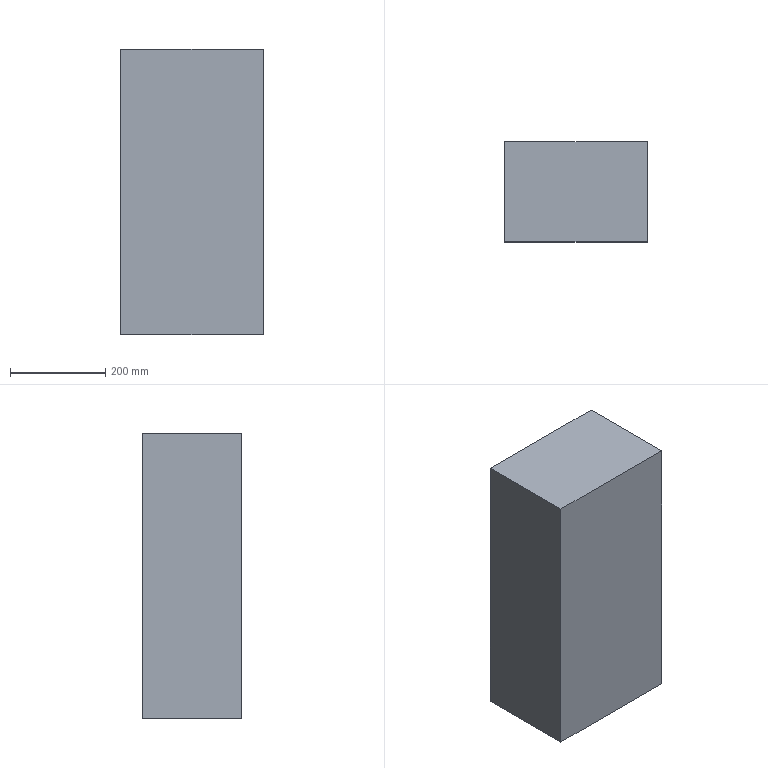Part | SolidWorks | features Extrusion 1 | 1 solid | 6 faces | box 300 x 210 x 600 mm | volume 37800000 mm3 | plane 6
STEP:
#1=CARTESIAN_POINT('',(150.,-105.,0.));
#2=VERTEX_POINT('',#1);
#3=CARTESIAN_POINT('',(150.,105.,0.));
#4=VERTEX_POINT('',#3);
#5=CARTESIAN_POINT('',(150.,105.,0.));
#6=DIRECTION('',(0.,1.,0.));
#7=VECTOR('',#6,1000.);
#8=LINE('',#5,#7);
#9=EDGE_CURVE('',#2,#4,#8,.T.);
#10=ORIENTED_EDGE('',*,*,#9,.T.);
#11=CARTESIAN_POINT('',(150.,105.,600.));
#12=VERTEX_POINT('',#11);
#13=CARTESIAN_POINT('',(150.,105.,600.));
#14=DIRECTION('',(0.,0.,-1.));
#15=VECTOR('',#14,1000.);
#16=LINE('',#13,#15);
#17=EDGE_CURVE('',#12,#4,#16,.T.);
#18=ORIENTED_EDGE('',*,*,#17,.F.);
#19=CARTESIAN_POINT('',(150.,-105.,600.));
#20=VERTEX_POINT('',#19);
#21=CARTESIAN_POINT('',(150.,105.,600.));
#22=DIRECTION('',(0.,1.,0.));
#23=VECTOR('',#22,1000.);
#24=LINE('',#21,#23);
#25=EDGE_CURVE('',#20,#12,#24,.T.);
#26=ORIENTED_EDGE('',*,*,#25,.F.);
#27=CARTESIAN_POINT('',(150.,-105.,600.));
#28=DIRECTION('',(0.,0.,-1.));
#29=VECTOR('',#28,1000.);
#30=LINE('',#27,#29);
#31=EDGE_CURVE('',#20,#2,#30,.T.);
#32=ORIENTED_EDGE('',*,*,#31,.T.);
#33=EDGE_LOOP('',(#10,#18,#26,#32));
#34=FACE_OUTER_BOUND('',#33,.T.);
#35=CARTESIAN_POINT('',(150.,105.,600.));
#36=DIRECTION('',(-1.,0.,0.));
#37=DIRECTION('',(0.,0.,1.));
#38=AXIS2_PLACEMENT_3D('',#35,#36,#37);
#39=PLANE('',#38);
#40=ADVANCED_FACE('',(#34),#39,.F.);
#41=CARTESIAN_POINT('',(-150.,105.,0.));
#42=VERTEX_POINT('',#41);
#43=CARTESIAN_POINT('',(-150.,105.,0.));
#44=DIRECTION('',(-1.,0.,0.));
#45=VECTOR('',#44,1000.);
#46=LINE('',#43,#45);
#47=EDGE_CURVE('',#4,#42,#46,.T.);
#48=ORIENTED_EDGE('',*,*,#47,.T.);
#49=CARTESIAN_POINT('',(-150.,105.,600.));
#50=VERTEX_POINT('',#49);
#51=CARTESIAN_POINT('',(-150.,105.,600.));
#52=DIRECTION('',(0.,0.,-1.));
#53=VECTOR('',#52,1000.);
#54=LINE('',#51,#53);
#55=EDGE_CURVE('',#50,#42,#54,.T.);
#56=ORIENTED_EDGE('',*,*,#55,.F.);
#57=CARTESIAN_POINT('',(-150.,105.,600.));
#58=DIRECTION('',(-1.,0.,0.));
#59=VECTOR('',#58,1000.);
#60=LINE('',#57,#59);
#61=EDGE_CURVE('',#12,#50,#60,.T.);
#62=ORIENTED_EDGE('',*,*,#61,.F.);
#63=ORIENTED_EDGE('',*,*,#17,.T.);
#64=EDGE_LOOP('',(#48,#56,#62,#63));
#65=FACE_OUTER_BOUND('',#64,.T.);
#66=CARTESIAN_POINT('',(-150.,105.,600.));
#67=DIRECTION('',(0.,-1.,0.));
#68=DIRECTION('',(0.,0.,-1.));
#69=AXIS2_PLACEMENT_3D('',#66,#67,#68);
#70=PLANE('',#69);
#71=ADVANCED_FACE('',(#65),#70,.F.);
#72=CARTESIAN_POINT('',(-150.,-105.,0.));
#73=VERTEX_POINT('',#72);
#74=CARTESIAN_POINT('',(-150.,105.,0.));
#75=DIRECTION('',(0.,-1.,0.));
#76=VECTOR('',#75,1000.);
#77=LINE('',#74,#76);
#78=EDGE_CURVE('',#42,#73,#77,.T.);
#79=ORIENTED_EDGE('',*,*,#78,.T.);
#80=CARTESIAN_POINT('',(-150.,-105.,600.));
#81=VERTEX_POINT('',#80);
#82=CARTESIAN_POINT('',(-150.,-105.,600.));
#83=DIRECTION('',(0.,0.,-1.));
#84=VECTOR('',#83,1000.);
#85=LINE('',#82,#84);
#86=EDGE_CURVE('',#81,#73,#85,.T.);
#87=ORIENTED_EDGE('',*,*,#86,.F.);
#88=CARTESIAN_POINT('',(-150.,105.,600.));
#89=DIRECTION('',(0.,-1.,0.));
#90=VECTOR('',#89,1000.);
#91=LINE('',#88,#90);
#92=EDGE_CURVE('',#50,#81,#91,.T.);
#93=ORIENTED_EDGE('',*,*,#92,.F.);
#94=ORIENTED_EDGE('',*,*,#55,.T.);
#95=EDGE_LOOP('',(#79,#87,#93,#94));
#96=FACE_OUTER_BOUND('',#95,.T.);
#97=CARTESIAN_POINT('',(-150.,105.,600.));
#98=DIRECTION('',(1.,0.,0.));
#99=DIRECTION('',(0.,1.,0.));
#100=AXIS2_PLACEMENT_3D('',#97,#98,#99);
#101=PLANE('',#100);
#102=ADVANCED_FACE('',(#96),#101,.F.);
#103=CARTESIAN_POINT('',(-150.,-105.,0.));
#104=DIRECTION('',(1.,0.,0.));
#105=VECTOR('',#104,1000.);
#106=LINE('',#103,#105);
#107=EDGE_CURVE('',#73,#2,#106,.T.);
#108=ORIENTED_EDGE('',*,*,#107,.T.);
#109=ORIENTED_EDGE('',*,*,#31,.F.);
#110=CARTESIAN_POINT('',(-150.,-105.,600.));
#111=DIRECTION('',(1.,0.,0.));
#112=VECTOR('',#111,1000.);
#113=LINE('',#110,#112);
#114=EDGE_CURVE('',#81,#20,#113,.T.);
#115=ORIENTED_EDGE('',*,*,#114,.F.);
#116=ORIENTED_EDGE('',*,*,#86,.T.);
#117=EDGE_LOOP('',(#108,#109,#115,#116));
#118=FACE_OUTER_BOUND('',#117,.T.);
#119=CARTESIAN_POINT('',(-150.,-105.,600.));
#120=DIRECTION('',(0.,1.,0.));
#121=DIRECTION('',(0.,0.,1.));
#122=AXIS2_PLACEMENT_3D('',#119,#120,#121);
#123=PLANE('',#122);
#124=ADVANCED_FACE('',(#118),#123,.F.);
#125=ORIENTED_EDGE('',*,*,#25,.T.);
#126=ORIENTED_EDGE('',*,*,#61,.T.);
#127=ORIENTED_EDGE('',*,*,#92,.T.);
#128=ORIENTED_EDGE('',*,*,#114,.T.);
#129=EDGE_LOOP('',(#125,#126,#127,#128));
#130=FACE_OUTER_BOUND('',#129,.T.);
#131=CARTESIAN_POINT('',(0.,0.,600.));
#132=DIRECTION('',(0.,0.,1.));
#133=DIRECTION('',(1.,0.,0.));
#134=AXIS2_PLACEMENT_3D('',#131,#132,#133);
#135=PLANE('',#134);
#136=ADVANCED_FACE('',(#130),#135,.T.);
#137=ORIENTED_EDGE('',*,*,#9,.F.);
#138=ORIENTED_EDGE('',*,*,#107,.F.);
#139=ORIENTED_EDGE('',*,*,#78,.F.);
#140=ORIENTED_EDGE('',*,*,#47,.F.);
#141=EDGE_LOOP('',(#137,#138,#139,#140));
#142=FACE_OUTER_BOUND('',#141,.T.);
#143=CARTESIAN_POINT('',(0.,0.,0.));
#144=DIRECTION('',(0.,0.,1.));
#145=DIRECTION('',(1.,0.,0.));
#146=AXIS2_PLACEMENT_3D('',#143,#144,#145);
#147=PLANE('',#146);
#148=ADVANCED_FACE('',(#142),#147,.F.);
#149=CLOSED_SHELL('',(#40,#71,#102,#124,#136,#148));
#150=MANIFOLD_SOLID_BREP('',#149);
#151=CARTESIAN_POINT('',(0.,0.,0.));
#152=DIRECTION('',(0.,0.,1.));
#153=DIRECTION('',(1.,0.,0.));
#154=AXIS2_PLACEMENT_3D('',#151,#152,#153);
#155=(LENGTH_UNIT()NAMED_UNIT(*)SI_UNIT(.MILLI.,.METRE.));
#156=UNCERTAINTY_MEASURE_WITH_UNIT(LENGTH_MEASURE(0.00001),#155,'','');
#157=(NAMED_UNIT(*)PLANE_ANGLE_UNIT()SI_UNIT($,.RADIAN.));
#158=(NAMED_UNIT(*)SI_UNIT($,.STERADIAN.)SOLID_ANGLE_UNIT());
#159=(GEOMETRIC_REPRESENTATION_CONTEXT(3)GLOBAL_UNCERTAINTY_ASSIGNED_CONTEXT((#156))GLOBAL_UNIT_ASSIGNED_CONTEXT((#155,#157,#158))REPRESENTATION_CONTEXT('',''));
#160=ADVANCED_BREP_SHAPE_REPRESENTATION('',(#150,#154),#159);